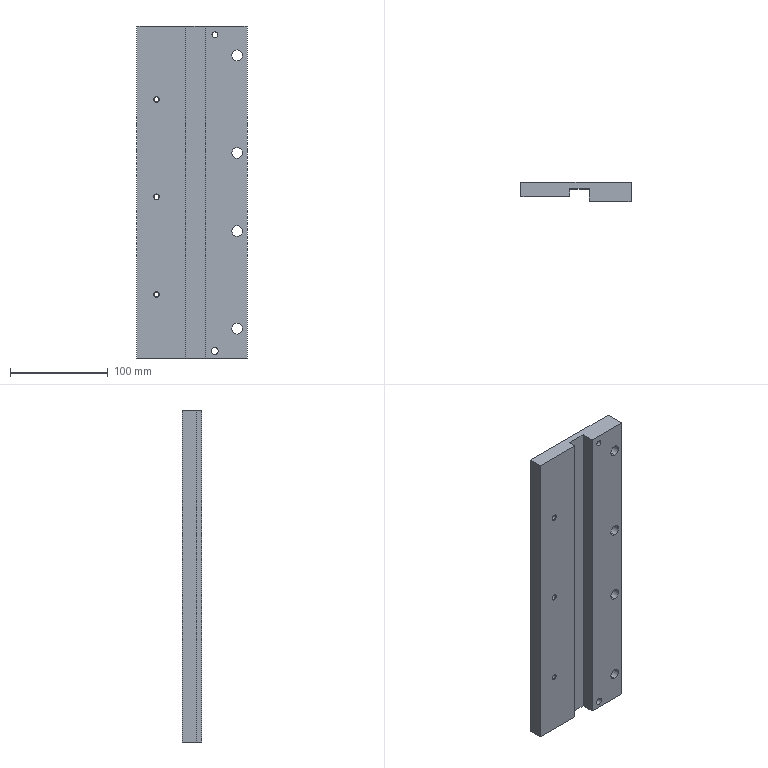Part | STEP file | 1 solid | 54 faces | box 112.747 x 19.5 x 340 mm | volume 560080 mm3 | cylinder 26 | cone 14 | plane 14 | commonest cylinder face diameters 11 x8 18 x8 5 x6 5.96 x2 7 x2